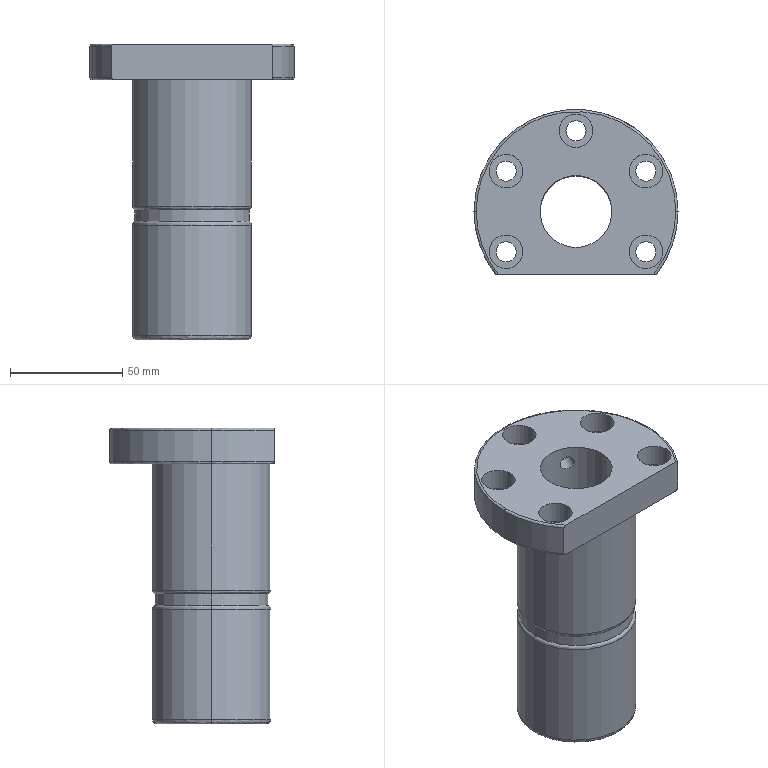Part | STEP file | 45LFDDC Lead Screw Seat 8M | 1 solid | 61 faces | box 91 x 73.5 x 132 mm | volume 225854 mm3 | cylinder 37 | spline 12 | plane 10 | cone 2 | commonest cylinder face diameters 9 x10 15 x10 53 x4 91 x3 6.5 x2 6.8 x2